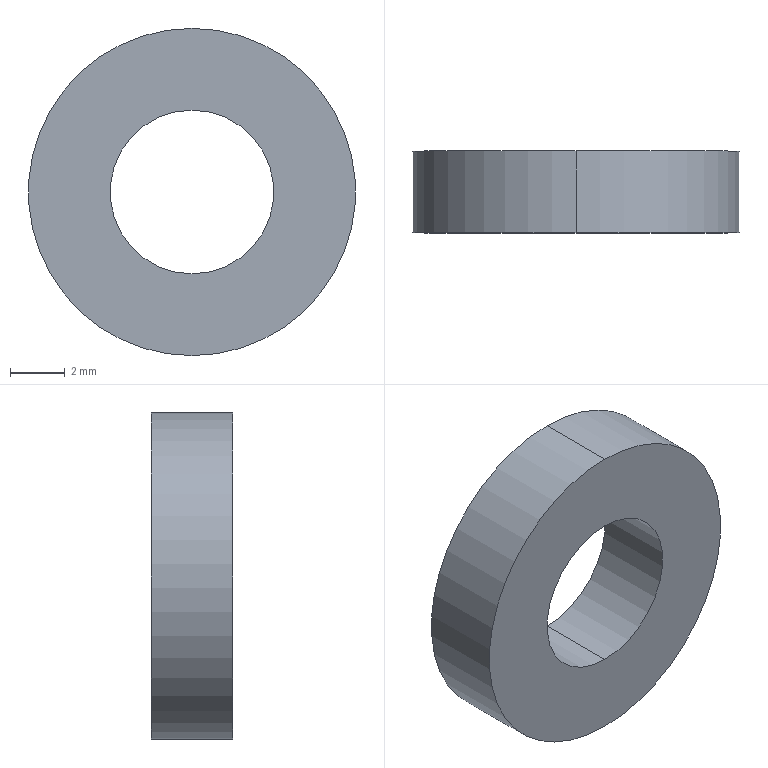Part | SolidWorks | features BaseBody 1 | 1 solid | 6 faces | box 12 x 3 x 12 mm | volume 254.469 mm3 | cylinder 4 | plane 2 | commonest cylinder face diameters 6 x2 12 x2
STEP:
#1=CARTESIAN_POINT('',(0.,3.,-6.));
#2=VERTEX_POINT('',#1);
#3=CARTESIAN_POINT('',(0.,3.,6.));
#4=VERTEX_POINT('',#3);
#5=CARTESIAN_POINT('',(0.,3.,0.));
#6=DIRECTION('',(0.,-1.,0.));
#7=DIRECTION('',(0.,0.,-1.));
#8=AXIS2_PLACEMENT_3D('',#5,#6,#7);
#9=CIRCLE('',#8,6.);
#10=EDGE_CURVE('',#2,#4,#9,.T.);
#11=ORIENTED_EDGE('',*,*,#10,.T.);
#12=CARTESIAN_POINT('',(0.,0.,6.));
#13=VERTEX_POINT('',#12);
#14=CARTESIAN_POINT('',(0.,-3.,6.));
#15=DIRECTION('',(0.,-1.,0.));
#16=VECTOR('',#15,1000.);
#17=LINE('',#14,#16);
#18=EDGE_CURVE('',#4,#13,#17,.T.);
#19=ORIENTED_EDGE('',*,*,#18,.T.);
#20=CARTESIAN_POINT('',(0.,0.,-6.));
#21=VERTEX_POINT('',#20);
#22=CARTESIAN_POINT('',(0.,0.,0.));
#23=DIRECTION('',(0.,-1.,0.));
#24=DIRECTION('',(0.,0.,-1.));
#25=AXIS2_PLACEMENT_3D('',#22,#23,#24);
#26=CIRCLE('',#25,6.);
#27=EDGE_CURVE('',#21,#13,#26,.T.);
#28=ORIENTED_EDGE('',*,*,#27,.F.);
#29=CARTESIAN_POINT('',(0.,-3.,-6.));
#30=DIRECTION('',(0.,-1.,0.));
#31=VECTOR('',#30,1000.);
#32=LINE('',#29,#31);
#33=EDGE_CURVE('',#2,#21,#32,.T.);
#34=ORIENTED_EDGE('',*,*,#33,.F.);
#35=EDGE_LOOP('',(#11,#19,#28,#34));
#36=FACE_OUTER_BOUND('',#35,.T.);
#37=CARTESIAN_POINT('',(0.,-3.,0.));
#38=DIRECTION('',(0.,-1.,0.));
#39=DIRECTION('',(0.,0.,-1.));
#40=AXIS2_PLACEMENT_3D('',#37,#38,#39);
#41=CYLINDRICAL_SURFACE('',#40,6.);
#42=ADVANCED_FACE('',(#36),#41,.T.);
#43=CARTESIAN_POINT('',(0.,3.,3.));
#44=VERTEX_POINT('',#43);
#45=CARTESIAN_POINT('',(0.,3.,-3.));
#46=VERTEX_POINT('',#45);
#47=CARTESIAN_POINT('',(0.,3.,0.));
#48=DIRECTION('',(0.,-1.,0.));
#49=DIRECTION('',(0.,0.,-1.));
#50=AXIS2_PLACEMENT_3D('',#47,#48,#49);
#51=CIRCLE('',#50,3.);
#52=EDGE_CURVE('',#44,#46,#51,.T.);
#53=ORIENTED_EDGE('',*,*,#52,.F.);
#54=CARTESIAN_POINT('',(0.,0.,3.));
#55=VERTEX_POINT('',#54);
#56=CARTESIAN_POINT('',(0.,-3.,3.));
#57=DIRECTION('',(0.,-1.,0.));
#58=VECTOR('',#57,1000.);
#59=LINE('',#56,#58);
#60=EDGE_CURVE('',#44,#55,#59,.T.);
#61=ORIENTED_EDGE('',*,*,#60,.T.);
#62=CARTESIAN_POINT('',(0.,0.,-3.));
#63=VERTEX_POINT('',#62);
#64=CARTESIAN_POINT('',(0.,0.,0.));
#65=DIRECTION('',(0.,-1.,0.));
#66=DIRECTION('',(0.,0.,-1.));
#67=AXIS2_PLACEMENT_3D('',#64,#65,#66);
#68=CIRCLE('',#67,3.);
#69=EDGE_CURVE('',#55,#63,#68,.T.);
#70=ORIENTED_EDGE('',*,*,#69,.T.);
#71=CARTESIAN_POINT('',(0.,-3.,-3.));
#72=DIRECTION('',(0.,-1.,0.));
#73=VECTOR('',#72,1000.);
#74=LINE('',#71,#73);
#75=EDGE_CURVE('',#46,#63,#74,.T.);
#76=ORIENTED_EDGE('',*,*,#75,.F.);
#77=EDGE_LOOP('',(#53,#61,#70,#76));
#78=FACE_OUTER_BOUND('',#77,.T.);
#79=CARTESIAN_POINT('',(0.,-3.,0.));
#80=DIRECTION('',(0.,-1.,0.));
#81=DIRECTION('',(0.,0.,-1.));
#82=AXIS2_PLACEMENT_3D('',#79,#80,#81);
#83=CYLINDRICAL_SURFACE('',#82,3.);
#84=ADVANCED_FACE('',(#78),#83,.F.);
#85=CARTESIAN_POINT('',(0.,3.,0.));
#86=DIRECTION('',(0.,-1.,0.));
#87=DIRECTION('',(0.,0.,-1.));
#88=AXIS2_PLACEMENT_3D('',#85,#86,#87);
#89=CIRCLE('',#88,3.);
#90=EDGE_CURVE('',#46,#44,#89,.T.);
#91=ORIENTED_EDGE('',*,*,#90,.T.);
#92=ORIENTED_EDGE('',*,*,#52,.T.);
#93=EDGE_LOOP('',(#91,#92));
#94=FACE_BOUND('',#93,.T.);
#95=ORIENTED_EDGE('',*,*,#10,.F.);
#96=CARTESIAN_POINT('',(0.,3.,0.));
#97=DIRECTION('',(0.,-1.,0.));
#98=DIRECTION('',(0.,0.,-1.));
#99=AXIS2_PLACEMENT_3D('',#96,#97,#98);
#100=CIRCLE('',#99,6.);
#101=EDGE_CURVE('',#4,#2,#100,.T.);
#102=ORIENTED_EDGE('',*,*,#101,.F.);
#103=EDGE_LOOP('',(#95,#102));
#104=FACE_OUTER_BOUND('',#103,.T.);
#105=CARTESIAN_POINT('',(6.,3.,0.));
#106=DIRECTION('',(0.,1.,0.));
#107=DIRECTION('',(0.,0.,1.));
#108=AXIS2_PLACEMENT_3D('',#105,#106,#107);
#109=PLANE('',#108);
#110=ADVANCED_FACE('',(#94,#104),#109,.T.);
#111=ORIENTED_EDGE('',*,*,#60,.F.);
#112=ORIENTED_EDGE('',*,*,#90,.F.);
#113=ORIENTED_EDGE('',*,*,#75,.T.);
#114=CARTESIAN_POINT('',(0.,0.,0.));
#115=DIRECTION('',(0.,-1.,0.));
#116=DIRECTION('',(0.,0.,-1.));
#117=AXIS2_PLACEMENT_3D('',#114,#115,#116);
#118=CIRCLE('',#117,3.);
#119=EDGE_CURVE('',#63,#55,#118,.T.);
#120=ORIENTED_EDGE('',*,*,#119,.T.);
#121=EDGE_LOOP('',(#111,#112,#113,#120));
#122=FACE_OUTER_BOUND('',#121,.T.);
#123=CARTESIAN_POINT('',(0.,-3.,0.));
#124=DIRECTION('',(0.,-1.,0.));
#125=DIRECTION('',(0.,0.,-1.));
#126=AXIS2_PLACEMENT_3D('',#123,#124,#125);
#127=CYLINDRICAL_SURFACE('',#126,3.);
#128=ADVANCED_FACE('',(#122),#127,.F.);
#129=ORIENTED_EDGE('',*,*,#18,.F.);
#130=ORIENTED_EDGE('',*,*,#101,.T.);
#131=ORIENTED_EDGE('',*,*,#33,.T.);
#132=CARTESIAN_POINT('',(0.,0.,0.));
#133=DIRECTION('',(0.,-1.,0.));
#134=DIRECTION('',(0.,0.,-1.));
#135=AXIS2_PLACEMENT_3D('',#132,#133,#134);
#136=CIRCLE('',#135,6.);
#137=EDGE_CURVE('',#13,#21,#136,.T.);
#138=ORIENTED_EDGE('',*,*,#137,.F.);
#139=EDGE_LOOP('',(#129,#130,#131,#138));
#140=FACE_OUTER_BOUND('',#139,.T.);
#141=CARTESIAN_POINT('',(0.,-3.,0.));
#142=DIRECTION('',(0.,-1.,0.));
#143=DIRECTION('',(0.,0.,-1.));
#144=AXIS2_PLACEMENT_3D('',#141,#142,#143);
#145=CYLINDRICAL_SURFACE('',#144,6.);
#146=ADVANCED_FACE('',(#140),#145,.T.);
#147=ORIENTED_EDGE('',*,*,#27,.T.);
#148=ORIENTED_EDGE('',*,*,#137,.T.);
#149=EDGE_LOOP('',(#147,#148));
#150=FACE_OUTER_BOUND('',#149,.T.);
#151=ORIENTED_EDGE('',*,*,#119,.F.);
#152=ORIENTED_EDGE('',*,*,#69,.F.);
#153=EDGE_LOOP('',(#151,#152));
#154=FACE_BOUND('',#153,.T.);
#155=CARTESIAN_POINT('',(3.,0.,0.));
#156=DIRECTION('',(0.,-1.,0.));
#157=DIRECTION('',(0.,0.,-1.));
#158=AXIS2_PLACEMENT_3D('',#155,#156,#157);
#159=PLANE('',#158);
#160=ADVANCED_FACE('',(#150,#154),#159,.T.);
#161=CLOSED_SHELL('',(#42,#84,#110,#128,#146,#160));
#162=MANIFOLD_SOLID_BREP('',#161);
#163=CARTESIAN_POINT('',(0.,0.,0.));
#164=DIRECTION('',(0.,0.,1.));
#165=DIRECTION('',(1.,0.,0.));
#166=AXIS2_PLACEMENT_3D('',#163,#164,#165);
#167=(LENGTH_UNIT()NAMED_UNIT(*)SI_UNIT(.MILLI.,.METRE.));
#168=UNCERTAINTY_MEASURE_WITH_UNIT(LENGTH_MEASURE(0.00001),#167,'','');
#169=(NAMED_UNIT(*)PLANE_ANGLE_UNIT()SI_UNIT($,.RADIAN.));
#170=(NAMED_UNIT(*)SI_UNIT($,.STERADIAN.)SOLID_ANGLE_UNIT());
#171=(GEOMETRIC_REPRESENTATION_CONTEXT(3)GLOBAL_UNCERTAINTY_ASSIGNED_CONTEXT((#168))GLOBAL_UNIT_ASSIGNED_CONTEXT((#167,#169,#170))REPRESENTATION_CONTEXT('',''));
#172=ADVANCED_BREP_SHAPE_REPRESENTATION('',(#162,#166),#171);